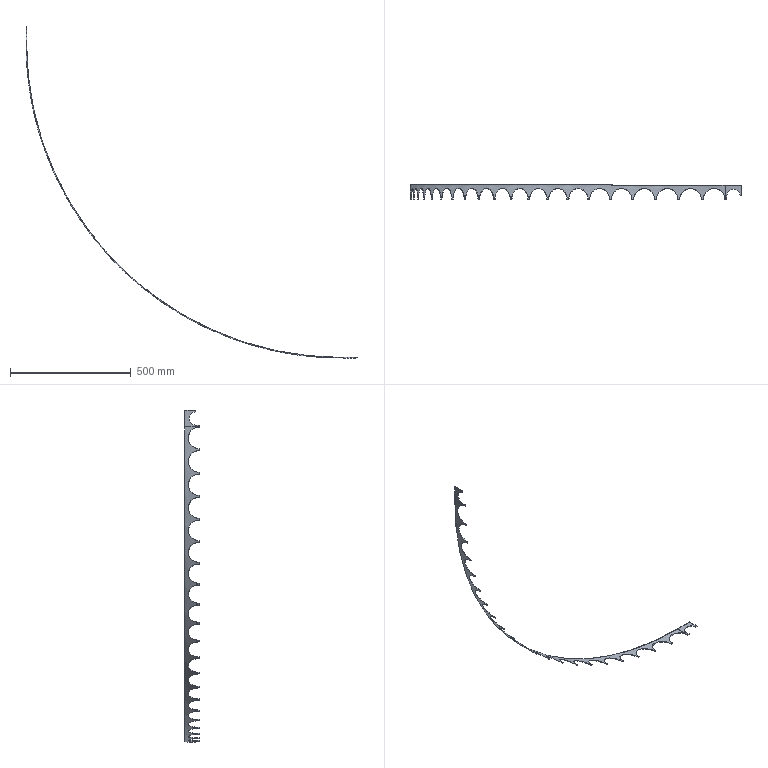Part | STEP file | covercurveroller-p11 | 1 solid | 58 faces | box 1374 x 60 x 1374 mm | volume 150099 mm3 | plane 31 | cylinder 14 | spline 13 | commonest cylinder face diameters 90 x11 55 x1 2602 x1 2607 x1